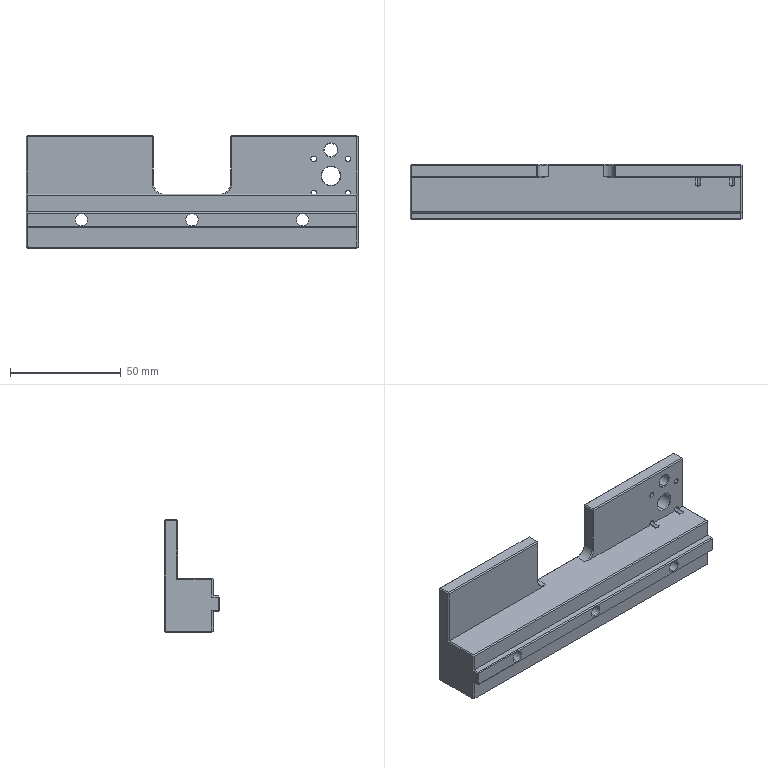Part | STEP file | BPSP-02-018 Fixture Locating Plate_Default | 1 solid | 101 faces | box 150 x 25 x 51 mm | volume 98863 mm3 | plane 65 | cylinder 26 | cone 10 | commonest cylinder face diameters 2.5 x8 10 x8 5.5 x6 6 x2 8.5 x2